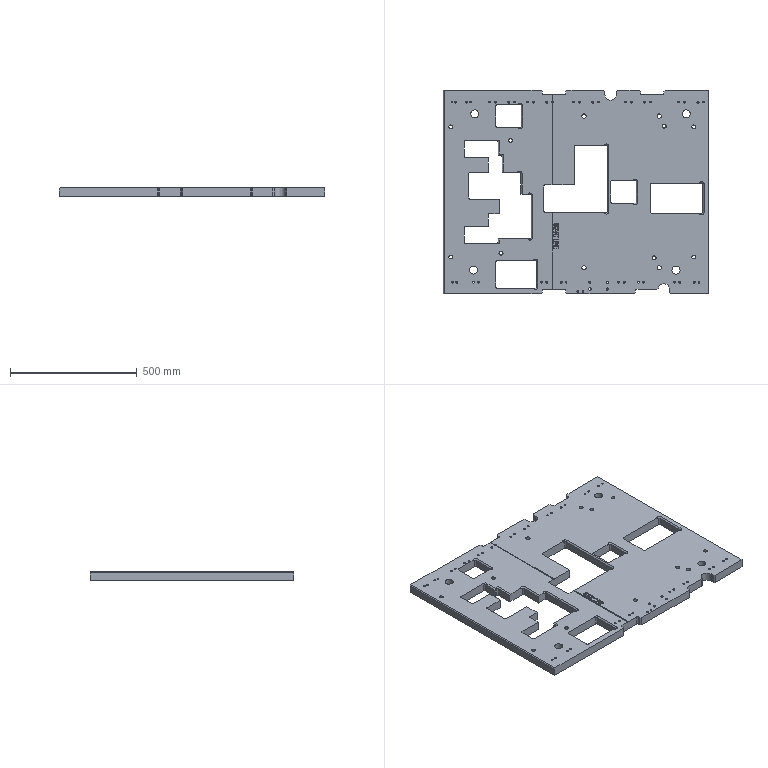Part | STEP file | lll_id10_x_t | 1 solid | 376 faces | box 1050 x 805 x 35 mm | volume 22562559 mm3 | plane 190 | cylinder 124 | cone 49 | other 13 | commonest cylinder face diameters 10 x40 8 x23 6.806 x18 6.8 x12 12 x7 14 x4